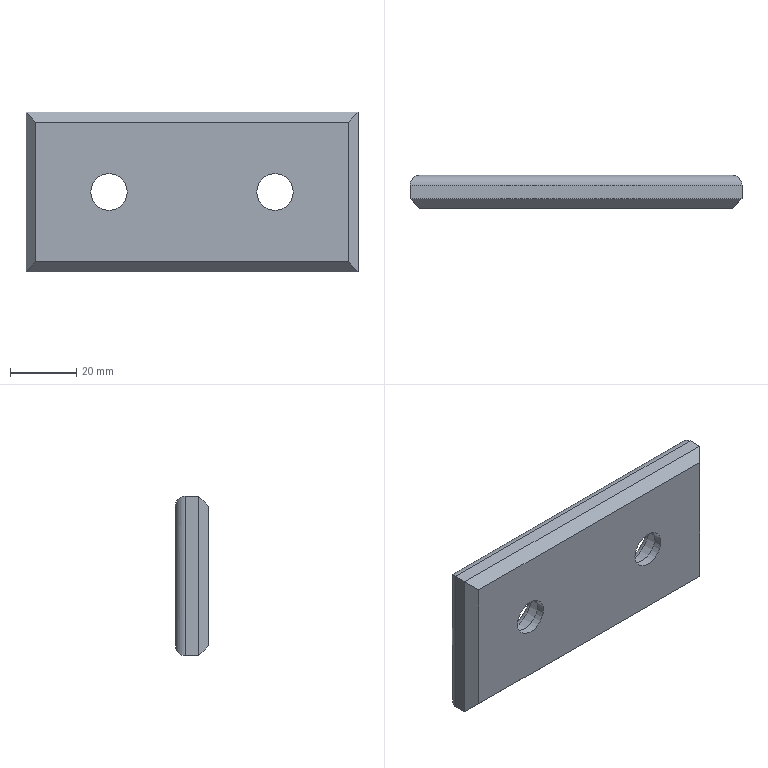Part | STEP file | lll_id4726_x_t | 1 solid | 22 faces | box 100 x 10 x 48 mm | volume 41960 mm3 | plane 12 | cylinder 8 | torus 2 | commonest cylinder face diameters 6 x4 11 x2 17.5 x2
STEP:
#1=CARTESIAN_POINT('',(1405.339,-363.359,5.));
#2=VERTEX_POINT('',#1);
#3=CARTESIAN_POINT('',(1405.339,-359.359,5.));
#4=VERTEX_POINT('',#3);
#5=CARTESIAN_POINT('',(1405.339,-361.359,5.));
#6=DIRECTION('',(0.,1.,0.));
#7=VECTOR('',#6,1.);
#8=LINE('',#5,#7);
#9=EDGE_CURVE('',#2,#4,#8,.T.);
#10=ORIENTED_EDGE('',*,*,#9,.T.);
#11=CARTESIAN_POINT('',(1305.339,-359.359,5.));
#12=VERTEX_POINT('',#11);
#13=CARTESIAN_POINT('',(1305.339,-359.359,5.));
#14=DIRECTION('',(-1.,0.,0.));
#15=VECTOR('',#14,1.);
#16=LINE('',#13,#15);
#17=EDGE_CURVE('',#4,#12,#16,.T.);
#18=ORIENTED_EDGE('',*,*,#17,.T.);
#19=CARTESIAN_POINT('',(1305.339,-363.359,5.));
#20=VERTEX_POINT('',#19);
#21=CARTESIAN_POINT('',(1305.339,-361.359,5.));
#22=DIRECTION('',(0.,-1.,0.));
#23=VECTOR('',#22,1.);
#24=LINE('',#21,#23);
#25=EDGE_CURVE('',#12,#20,#24,.T.);
#26=ORIENTED_EDGE('',*,*,#25,.T.);
#27=CARTESIAN_POINT('',(1305.339,-363.359,5.));
#28=DIRECTION('',(1.,0.,0.));
#29=VECTOR('',#28,1.);
#30=LINE('',#27,#29);
#31=EDGE_CURVE('',#20,#2,#30,.T.);
#32=ORIENTED_EDGE('',*,*,#31,.T.);
#33=EDGE_LOOP('',(#10,#18,#26,#32));
#34=FACE_OUTER_BOUND('',#33,.T.);
#35=CARTESIAN_POINT('',(1305.339,-361.359,5.));
#36=DIRECTION('',(0.,0.,1.));
#37=DIRECTION('',(-1.,0.,0.));
#38=AXIS2_PLACEMENT_3D('',#35,#36,#37);
#39=PLANE('',#38);
#40=ADVANCED_FACE('',(#34),#39,.T.);
#41=CARTESIAN_POINT('',(1405.339,-359.359,-43.));
#42=VERTEX_POINT('',#41);
#43=CARTESIAN_POINT('',(1405.339,-363.359,-43.));
#44=VERTEX_POINT('',#43);
#45=CARTESIAN_POINT('',(1405.339,-361.359,-43.));
#46=DIRECTION('',(0.,-1.,0.));
#47=VECTOR('',#46,1.);
#48=LINE('',#45,#47);
#49=EDGE_CURVE('',#42,#44,#48,.T.);
#50=ORIENTED_EDGE('',*,*,#49,.F.);
#51=CARTESIAN_POINT('',(1405.339,-359.359,-19.));
#52=DIRECTION('',(0.,0.,1.));
#53=VECTOR('',#52,1.);
#54=LINE('',#51,#53);
#55=EDGE_CURVE('',#42,#4,#54,.T.);
#56=ORIENTED_EDGE('',*,*,#55,.T.);
#57=ORIENTED_EDGE('',*,*,#9,.F.);
#58=CARTESIAN_POINT('',(1405.339,-363.359,-19.));
#59=DIRECTION('',(0.,0.,-1.));
#60=VECTOR('',#59,1.);
#61=LINE('',#58,#60);
#62=EDGE_CURVE('',#2,#44,#61,.T.);
#63=ORIENTED_EDGE('',*,*,#62,.T.);
#64=EDGE_LOOP('',(#50,#56,#57,#63));
#65=FACE_OUTER_BOUND('',#64,.T.);
#66=CARTESIAN_POINT('',(1405.339,-361.359,-19.));
#67=DIRECTION('',(1.,0.,0.));
#68=DIRECTION('',(0.,0.,1.));
#69=AXIS2_PLACEMENT_3D('',#66,#67,#68);
#70=PLANE('',#69);
#71=ADVANCED_FACE('',(#65),#70,.T.);
#72=CARTESIAN_POINT('',(1369.589,-356.359,-19.));
#73=VERTEX_POINT('',#72);
#74=CARTESIAN_POINT('',(1380.339,-356.359,-19.));
#75=DIRECTION('',(0.,-1.,0.));
#76=DIRECTION('',(-1.,0.,0.));
#77=AXIS2_PLACEMENT_3D('',#74,#75,#76);
#78=CIRCLE('',#77,10.75);
#79=EDGE_CURVE('',#73,#73,#78,.T.);
#80=ORIENTED_EDGE('',*,*,#79,.T.);
#81=EDGE_LOOP('',(#80));
#82=FACE_BOUND('',#81,.T.);
#83=CARTESIAN_POINT('',(1319.589,-356.359,-19.));
#84=VERTEX_POINT('',#83);
#85=CARTESIAN_POINT('',(1330.339,-356.359,-19.));
#86=DIRECTION('',(0.,-1.,0.));
#87=DIRECTION('',(-1.,0.,0.));
#88=AXIS2_PLACEMENT_3D('',#85,#86,#87);
#89=CIRCLE('',#88,10.75);
#90=EDGE_CURVE('',#84,#84,#89,.T.);
#91=ORIENTED_EDGE('',*,*,#90,.T.);
#92=EDGE_LOOP('',(#91));
#93=FACE_BOUND('',#92,.T.);
#94=CARTESIAN_POINT('',(1402.339,-356.359,-40.));
#95=VERTEX_POINT('',#94);
#96=CARTESIAN_POINT('',(1308.339,-356.359,-40.));
#97=VERTEX_POINT('',#96);
#98=CARTESIAN_POINT('',(1305.339,-356.359,-40.));
#99=DIRECTION('',(-1.,0.,0.));
#100=VECTOR('',#99,1.);
#101=LINE('',#98,#100);
#102=EDGE_CURVE('',#95,#97,#101,.T.);
#103=ORIENTED_EDGE('',*,*,#102,.T.);
#104=CARTESIAN_POINT('',(1308.339,-356.359,2.));
#105=VERTEX_POINT('',#104);
#106=CARTESIAN_POINT('',(1308.339,-356.359,-19.));
#107=DIRECTION('',(0.,0.,1.));
#108=VECTOR('',#107,1.);
#109=LINE('',#106,#108);
#110=EDGE_CURVE('',#97,#105,#109,.T.);
#111=ORIENTED_EDGE('',*,*,#110,.T.);
#112=CARTESIAN_POINT('',(1402.339,-356.359,2.));
#113=VERTEX_POINT('',#112);
#114=CARTESIAN_POINT('',(1305.339,-356.359,2.));
#115=DIRECTION('',(1.,0.,0.));
#116=VECTOR('',#115,1.);
#117=LINE('',#114,#116);
#118=EDGE_CURVE('',#105,#113,#117,.T.);
#119=ORIENTED_EDGE('',*,*,#118,.T.);
#120=CARTESIAN_POINT('',(1402.339,-356.359,-19.));
#121=DIRECTION('',(0.,0.,-1.));
#122=VECTOR('',#121,1.);
#123=LINE('',#120,#122);
#124=EDGE_CURVE('',#113,#95,#123,.T.);
#125=ORIENTED_EDGE('',*,*,#124,.T.);
#126=EDGE_LOOP('',(#103,#111,#119,#125));
#127=FACE_BOUND('',#126,.T.);
#128=CARTESIAN_POINT('',(1305.339,-356.359,-19.));
#129=DIRECTION('',(0.,1.,0.));
#130=DIRECTION('',(-1.,0.,0.));
#131=AXIS2_PLACEMENT_3D('',#128,#129,#130);
#132=PLANE('',#131);
#133=ADVANCED_FACE('',(#82,#93,#127),#132,.T.);
#134=CARTESIAN_POINT('',(1305.339,-363.359,-43.));
#135=VERTEX_POINT('',#134);
#136=CARTESIAN_POINT('',(1305.339,-359.359,-43.));
#137=VERTEX_POINT('',#136);
#138=CARTESIAN_POINT('',(1305.339,-361.359,-43.));
#139=DIRECTION('',(0.,1.,0.));
#140=VECTOR('',#139,1.);
#141=LINE('',#138,#140);
#142=EDGE_CURVE('',#135,#137,#141,.T.);
#143=ORIENTED_EDGE('',*,*,#142,.T.);
#144=CARTESIAN_POINT('',(1305.339,-359.359,-43.));
#145=DIRECTION('',(1.,0.,0.));
#146=VECTOR('',#145,1.);
#147=LINE('',#144,#146);
#148=EDGE_CURVE('',#137,#42,#147,.T.);
#149=ORIENTED_EDGE('',*,*,#148,.T.);
#150=ORIENTED_EDGE('',*,*,#49,.T.);
#151=CARTESIAN_POINT('',(1305.339,-363.359,-43.));
#152=DIRECTION('',(-1.,0.,0.));
#153=VECTOR('',#152,1.);
#154=LINE('',#151,#153);
#155=EDGE_CURVE('',#44,#135,#154,.T.);
#156=ORIENTED_EDGE('',*,*,#155,.T.);
#157=EDGE_LOOP('',(#143,#149,#150,#156));
#158=FACE_OUTER_BOUND('',#157,.T.);
#159=CARTESIAN_POINT('',(1305.339,-361.359,-43.));
#160=DIRECTION('',(0.,0.,-1.));
#161=DIRECTION('',(1.,0.,0.));
#162=AXIS2_PLACEMENT_3D('',#159,#160,#161);
#163=PLANE('',#162);
#164=ADVANCED_FACE('',(#158),#163,.T.);
#165=CARTESIAN_POINT('',(1374.839,-366.359,-19.));
#166=VERTEX_POINT('',#165);
#167=CARTESIAN_POINT('',(1380.339,-366.359,-19.));
#168=DIRECTION('',(0.,1.,0.));
#169=DIRECTION('',(-1.,0.,0.));
#170=AXIS2_PLACEMENT_3D('',#167,#168,#169);
#171=CIRCLE('',#170,5.5);
#172=EDGE_CURVE('',#166,#166,#171,.T.);
#173=ORIENTED_EDGE('',*,*,#172,.T.);
#174=EDGE_LOOP('',(#173));
#175=FACE_BOUND('',#174,.T.);
#176=CARTESIAN_POINT('',(1324.839,-366.359,-19.));
#177=VERTEX_POINT('',#176);
#178=CARTESIAN_POINT('',(1330.339,-366.359,-19.));
#179=DIRECTION('',(0.,1.,0.));
#180=DIRECTION('',(-1.,0.,0.));
#181=AXIS2_PLACEMENT_3D('',#178,#179,#180);
#182=CIRCLE('',#181,5.5);
#183=EDGE_CURVE('',#177,#177,#182,.T.);
#184=ORIENTED_EDGE('',*,*,#183,.T.);
#185=EDGE_LOOP('',(#184));
#186=FACE_BOUND('',#185,.T.);
#187=CARTESIAN_POINT('',(1402.339,-366.359,2.));
#188=VERTEX_POINT('',#187);
#189=CARTESIAN_POINT('',(1308.339,-366.359,2.));
#190=VERTEX_POINT('',#189);
#191=CARTESIAN_POINT('',(1305.339,-366.359,2.));
#192=DIRECTION('',(-1.,0.,0.));
#193=VECTOR('',#192,1.);
#194=LINE('',#191,#193);
#195=EDGE_CURVE('',#188,#190,#194,.T.);
#196=ORIENTED_EDGE('',*,*,#195,.T.);
#197=CARTESIAN_POINT('',(1308.339,-366.359,-40.));
#198=VERTEX_POINT('',#197);
#199=CARTESIAN_POINT('',(1308.339,-366.359,-19.));
#200=DIRECTION('',(0.,0.,-1.));
#201=VECTOR('',#200,1.);
#202=LINE('',#199,#201);
#203=EDGE_CURVE('',#190,#198,#202,.T.);
#204=ORIENTED_EDGE('',*,*,#203,.T.);
#205=CARTESIAN_POINT('',(1402.339,-366.359,-40.));
#206=VERTEX_POINT('',#205);
#207=CARTESIAN_POINT('',(1305.339,-366.359,-40.));
#208=DIRECTION('',(1.,0.,0.));
#209=VECTOR('',#208,1.);
#210=LINE('',#207,#209);
#211=EDGE_CURVE('',#198,#206,#210,.T.);
#212=ORIENTED_EDGE('',*,*,#211,.T.);
#213=CARTESIAN_POINT('',(1402.339,-366.359,-19.));
#214=DIRECTION('',(0.,0.,1.));
#215=VECTOR('',#214,1.);
#216=LINE('',#213,#215);
#217=EDGE_CURVE('',#206,#188,#216,.T.);
#218=ORIENTED_EDGE('',*,*,#217,.T.);
#219=EDGE_LOOP('',(#196,#204,#212,#218));
#220=FACE_BOUND('',#219,.T.);
#221=CARTESIAN_POINT('',(1305.339,-366.359,-19.));
#222=DIRECTION('',(0.,-1.,0.));
#223=DIRECTION('',(1.,0.,0.));
#224=AXIS2_PLACEMENT_3D('',#221,#222,#223);
#225=PLANE('',#224);
#226=ADVANCED_FACE('',(#175,#186,#220),#225,.T.);
#227=ORIENTED_EDGE('',*,*,#25,.F.);
#228=CARTESIAN_POINT('',(1305.339,-359.359,-19.));
#229=DIRECTION('',(0.,0.,-1.));
#230=VECTOR('',#229,1.);
#231=LINE('',#228,#230);
#232=EDGE_CURVE('',#12,#137,#231,.T.);
#233=ORIENTED_EDGE('',*,*,#232,.T.);
#234=ORIENTED_EDGE('',*,*,#142,.F.);
#235=CARTESIAN_POINT('',(1305.339,-363.359,-19.));
#236=DIRECTION('',(0.,0.,1.));
#237=VECTOR('',#236,1.);
#238=LINE('',#235,#237);
#239=EDGE_CURVE('',#135,#20,#238,.T.);
#240=ORIENTED_EDGE('',*,*,#239,.T.);
#241=EDGE_LOOP('',(#227,#233,#234,#240));
#242=FACE_OUTER_BOUND('',#241,.T.);
#243=CARTESIAN_POINT('',(1305.339,-361.359,-19.));
#244=DIRECTION('',(-1.,0.,0.));
#245=DIRECTION('',(0.,0.,-1.));
#246=AXIS2_PLACEMENT_3D('',#243,#244,#245);
#247=PLANE('',#246);
#248=ADVANCED_FACE('',(#242),#247,.T.);
#249=CARTESIAN_POINT('',(1395.339,-373.359,-33.));
#250=DIRECTION('',(-0.5774,-0.5774,0.5774));
#251=VECTOR('',#250,1.);
#252=LINE('',#249,#251);
#253=EDGE_CURVE('',#44,#206,#252,.T.);
#254=ORIENTED_EDGE('',*,*,#253,.F.);
#255=ORIENTED_EDGE('',*,*,#62,.F.);
#256=CARTESIAN_POINT('',(1395.339,-373.359,-5.));
#257=DIRECTION('',(0.5774,0.5774,0.5774));
#258=VECTOR('',#257,1.);
#259=LINE('',#256,#258);
#260=EDGE_CURVE('',#188,#2,#259,.T.);
#261=ORIENTED_EDGE('',*,*,#260,.F.);
#262=ORIENTED_EDGE('',*,*,#217,.F.);
#263=EDGE_LOOP('',(#254,#255,#261,#262));
#264=FACE_OUTER_BOUND('',#263,.T.);
#265=CARTESIAN_POINT('',(1402.339,-366.359,-19.));
#266=DIRECTION('',(-0.7071,0.7071,0.));
#267=DIRECTION('',(-0.7071,-0.7071,0.));
#268=AXIS2_PLACEMENT_3D('',#265,#266,#267);
#269=PLANE('',#268);
#270=ADVANCED_FACE('',(#264),#269,.F.);
#271=ORIENTED_EDGE('',*,*,#260,.T.);
#272=ORIENTED_EDGE('',*,*,#31,.F.);
#273=CARTESIAN_POINT('',(1305.339,-363.359,5.));
#274=DIRECTION('',(-0.5774,0.5774,0.5774));
#275=VECTOR('',#274,1.);
#276=LINE('',#273,#275);
#277=EDGE_CURVE('',#190,#20,#276,.T.);
#278=ORIENTED_EDGE('',*,*,#277,.F.);
#279=ORIENTED_EDGE('',*,*,#195,.F.);
#280=EDGE_LOOP('',(#271,#272,#278,#279));
#281=FACE_OUTER_BOUND('',#280,.T.);
#282=CARTESIAN_POINT('',(1305.339,-363.359,5.));
#283=DIRECTION('',(0.,0.7071,-0.7071));
#284=DIRECTION('',(0.,0.7071,0.7071));
#285=AXIS2_PLACEMENT_3D('',#282,#283,#284);
#286=PLANE('',#285);
#287=ADVANCED_FACE('',(#281),#286,.F.);
#288=ORIENTED_EDGE('',*,*,#253,.T.);
#289=ORIENTED_EDGE('',*,*,#211,.F.);
#290=CARTESIAN_POINT('',(1307.339,-365.359,-41.));
#291=DIRECTION('',(0.5774,-0.5774,0.5774));
#292=VECTOR('',#291,1.);
#293=LINE('',#290,#292);
#294=EDGE_CURVE('',#135,#198,#293,.T.);
#295=ORIENTED_EDGE('',*,*,#294,.F.);
#296=ORIENTED_EDGE('',*,*,#155,.F.);
#297=EDGE_LOOP('',(#288,#289,#295,#296));
#298=FACE_OUTER_BOUND('',#297,.T.);
#299=CARTESIAN_POINT('',(1305.339,-366.359,-40.));
#300=DIRECTION('',(0.,0.7071,0.7071));
#301=DIRECTION('',(0.,-0.7071,0.7071));
#302=AXIS2_PLACEMENT_3D('',#299,#300,#301);
#303=PLANE('',#302);
#304=ADVANCED_FACE('',(#298),#303,.F.);
#305=ORIENTED_EDGE('',*,*,#277,.T.);
#306=ORIENTED_EDGE('',*,*,#239,.F.);
#307=ORIENTED_EDGE('',*,*,#294,.T.);
#308=ORIENTED_EDGE('',*,*,#203,.F.);
#309=EDGE_LOOP('',(#305,#306,#307,#308));
#310=FACE_OUTER_BOUND('',#309,.T.);
#311=CARTESIAN_POINT('',(1308.339,-366.359,-19.));
#312=DIRECTION('',(0.7071,0.7071,0.));
#313=DIRECTION('',(-0.7071,0.7071,0.));
#314=AXIS2_PLACEMENT_3D('',#311,#312,#313);
#315=PLANE('',#314);
#316=ADVANCED_FACE('',(#310),#315,.F.);
#317=CARTESIAN_POINT('',(1402.339,-359.359,2.));
#318=DIRECTION('',(-0.7071,0.,0.7071));
#319=DIRECTION('',(-0.7071,0.,-0.7071));
#320=AXIS2_PLACEMENT_3D('',#317,#318,#319);
#321=ELLIPSE('',#320,4.243,3.);
#322=EDGE_CURVE('',#4,#113,#321,.T.);
#323=ORIENTED_EDGE('',*,*,#322,.F.);
#324=ORIENTED_EDGE('',*,*,#55,.F.);
#325=CARTESIAN_POINT('',(1402.339,-359.359,-40.));
#326=DIRECTION('',(-0.7071,0.,-0.7071));
#327=DIRECTION('',(0.7071,0.,-0.7071));
#328=AXIS2_PLACEMENT_3D('',#325,#326,#327);
#329=ELLIPSE('',#328,4.243,3.);
#330=EDGE_CURVE('',#95,#42,#329,.T.);
#331=ORIENTED_EDGE('',*,*,#330,.F.);
#332=ORIENTED_EDGE('',*,*,#124,.F.);
#333=EDGE_LOOP('',(#323,#324,#331,#332));
#334=FACE_OUTER_BOUND('',#333,.T.);
#335=CARTESIAN_POINT('',(1402.339,-359.359,-19.));
#336=DIRECTION('',(0.,0.,-1.));
#337=DIRECTION('',(1.,0.,0.));
#338=AXIS2_PLACEMENT_3D('',#335,#336,#337);
#339=CYLINDRICAL_SURFACE('',#338,3.);
#340=ADVANCED_FACE('',(#334),#339,.T.);
#341=ORIENTED_EDGE('',*,*,#330,.T.);
#342=ORIENTED_EDGE('',*,*,#148,.F.);
#343=CARTESIAN_POINT('',(1308.339,-359.359,-40.));
#344=DIRECTION('',(-0.7071,0.,0.7071));
#345=DIRECTION('',(0.7071,0.,0.7071));
#346=AXIS2_PLACEMENT_3D('',#343,#344,#345);
#347=ELLIPSE('',#346,4.243,3.);
#348=EDGE_CURVE('',#97,#137,#347,.T.);
#349=ORIENTED_EDGE('',*,*,#348,.F.);
#350=ORIENTED_EDGE('',*,*,#102,.F.);
#351=EDGE_LOOP('',(#341,#342,#349,#350));
#352=FACE_OUTER_BOUND('',#351,.T.);
#353=CARTESIAN_POINT('',(1305.339,-359.359,-40.));
#354=DIRECTION('',(1.,0.,0.));
#355=DIRECTION('',(0.,0.,1.));
#356=AXIS2_PLACEMENT_3D('',#353,#354,#355);
#357=CYLINDRICAL_SURFACE('',#356,3.);
#358=ADVANCED_FACE('',(#352),#357,.T.);
#359=ORIENTED_EDGE('',*,*,#322,.T.);
#360=ORIENTED_EDGE('',*,*,#118,.F.);
#361=CARTESIAN_POINT('',(1308.339,-359.359,2.));
#362=DIRECTION('',(-0.7071,0.,-0.7071));
#363=DIRECTION('',(0.7071,0.,-0.7071));
#364=AXIS2_PLACEMENT_3D('',#361,#362,#363);
#365=ELLIPSE('',#364,4.243,3.);
#366=EDGE_CURVE('',#12,#105,#365,.T.);
#367=ORIENTED_EDGE('',*,*,#366,.F.);
#368=ORIENTED_EDGE('',*,*,#17,.F.);
#369=EDGE_LOOP('',(#359,#360,#367,#368));
#370=FACE_OUTER_BOUND('',#369,.T.);
#371=CARTESIAN_POINT('',(1305.339,-359.359,2.));
#372=DIRECTION('',(1.,0.,0.));
#373=DIRECTION('',(0.,0.,1.));
#374=AXIS2_PLACEMENT_3D('',#371,#372,#373);
#375=CYLINDRICAL_SURFACE('',#374,3.);
#376=ADVANCED_FACE('',(#370),#375,.T.);
#377=ORIENTED_EDGE('',*,*,#348,.T.);
#378=ORIENTED_EDGE('',*,*,#232,.F.);
#379=ORIENTED_EDGE('',*,*,#366,.T.);
#380=ORIENTED_EDGE('',*,*,#110,.F.);
#381=EDGE_LOOP('',(#377,#378,#379,#380));
#382=FACE_OUTER_BOUND('',#381,.T.);
#383=CARTESIAN_POINT('',(1308.339,-359.359,-19.));
#384=DIRECTION('',(0.,0.,1.));
#385=DIRECTION('',(-1.,0.,0.));
#386=AXIS2_PLACEMENT_3D('',#383,#384,#385);
#387=CYLINDRICAL_SURFACE('',#386,3.);
#388=ADVANCED_FACE('',(#382),#387,.T.);
#389=CARTESIAN_POINT('',(1335.839,-363.859,-19.));
#390=VERTEX_POINT('',#389);
#391=CARTESIAN_POINT('',(1330.339,-363.859,-19.));
#392=DIRECTION('',(0.,-1.,0.));
#393=DIRECTION('',(1.,0.,0.));
#394=AXIS2_PLACEMENT_3D('',#391,#392,#393);
#395=CIRCLE('',#394,5.5);
#396=EDGE_CURVE('',#390,#390,#395,.T.);
#397=ORIENTED_EDGE('',*,*,#396,.T.);
#398=EDGE_LOOP('',(#397));
#399=FACE_BOUND('',#398,.T.);
#400=CARTESIAN_POINT('',(1321.589,-363.859,-19.));
#401=VERTEX_POINT('',#400);
#402=CARTESIAN_POINT('',(1330.339,-363.859,-19.));
#403=DIRECTION('',(0.,-1.,0.));
#404=DIRECTION('',(-1.,0.,0.));
#405=AXIS2_PLACEMENT_3D('',#402,#403,#404);
#406=CIRCLE('',#405,8.75);
#407=EDGE_CURVE('',#401,#401,#406,.T.);
#408=ORIENTED_EDGE('',*,*,#407,.F.);
#409=EDGE_LOOP('',(#408));
#410=FACE_BOUND('',#409,.T.);
#411=CARTESIAN_POINT('',(1330.339,-363.859,-19.));
#412=DIRECTION('',(0.,-1.,0.));
#413=DIRECTION('',(1.,0.,0.));
#414=AXIS2_PLACEMENT_3D('',#411,#412,#413);
#415=PLANE('',#414);
#416=ADVANCED_FACE('',(#399,#410),#415,.F.);
#417=CARTESIAN_POINT('',(1321.589,-358.359,-19.));
#418=VERTEX_POINT('',#417);
#419=CARTESIAN_POINT('',(1330.339,-358.359,-19.));
#420=DIRECTION('',(0.,1.,0.));
#421=DIRECTION('',(-1.,0.,0.));
#422=AXIS2_PLACEMENT_3D('',#419,#420,#421);
#423=CIRCLE('',#422,8.75);
#424=EDGE_CURVE('',#418,#418,#423,.T.);
#425=ORIENTED_EDGE('',*,*,#424,.T.);
#426=EDGE_LOOP('',(#425));
#427=FACE_BOUND('',#426,.T.);
#428=ORIENTED_EDGE('',*,*,#407,.T.);
#429=EDGE_LOOP('',(#428));
#430=FACE_BOUND('',#429,.T.);
#431=CARTESIAN_POINT('',(1330.339,-356.359,-19.));
#432=DIRECTION('',(0.,-1.,0.));
#433=DIRECTION('',(1.,0.,0.));
#434=AXIS2_PLACEMENT_3D('',#431,#432,#433);
#435=CYLINDRICAL_SURFACE('',#434,8.75);
#436=ADVANCED_FACE('',(#427,#430),#435,.F.);
#437=ORIENTED_EDGE('',*,*,#183,.F.);
#438=EDGE_LOOP('',(#437));
#439=FACE_BOUND('',#438,.T.);
#440=ORIENTED_EDGE('',*,*,#396,.F.);
#441=EDGE_LOOP('',(#440));
#442=FACE_BOUND('',#441,.T.);
#443=CARTESIAN_POINT('',(1330.339,-356.359,-19.));
#444=DIRECTION('',(0.,-1.,0.));
#445=DIRECTION('',(1.,0.,0.));
#446=AXIS2_PLACEMENT_3D('',#443,#444,#445);
#447=CYLINDRICAL_SURFACE('',#446,5.5);
#448=ADVANCED_FACE('',(#439,#442),#447,.F.);
#449=CARTESIAN_POINT('',(1385.839,-363.859,-19.));
#450=VERTEX_POINT('',#449);
#451=CARTESIAN_POINT('',(1380.339,-363.859,-19.));
#452=DIRECTION('',(0.,-1.,0.));
#453=DIRECTION('',(1.,0.,0.));
#454=AXIS2_PLACEMENT_3D('',#451,#452,#453);
#455=CIRCLE('',#454,5.5);
#456=EDGE_CURVE('',#450,#450,#455,.T.);
#457=ORIENTED_EDGE('',*,*,#456,.T.);
#458=EDGE_LOOP('',(#457));
#459=FACE_BOUND('',#458,.T.);
#460=CARTESIAN_POINT('',(1371.589,-363.859,-19.));
#461=VERTEX_POINT('',#460);
#462=CARTESIAN_POINT('',(1380.339,-363.859,-19.));
#463=DIRECTION('',(0.,-1.,0.));
#464=DIRECTION('',(-1.,0.,0.));
#465=AXIS2_PLACEMENT_3D('',#462,#463,#464);
#466=CIRCLE('',#465,8.75);
#467=EDGE_CURVE('',#461,#461,#466,.T.);
#468=ORIENTED_EDGE('',*,*,#467,.F.);
#469=EDGE_LOOP('',(#468));
#470=FACE_BOUND('',#469,.T.);
#471=CARTESIAN_POINT('',(1380.339,-363.859,-19.));
#472=DIRECTION('',(0.,-1.,0.));
#473=DIRECTION('',(1.,0.,0.));
#474=AXIS2_PLACEMENT_3D('',#471,#472,#473);
#475=PLANE('',#474);
#476=ADVANCED_FACE('',(#459,#470),#475,.F.);
#477=CARTESIAN_POINT('',(1371.589,-358.359,-19.));
#478=VERTEX_POINT('',#477);
#479=CARTESIAN_POINT('',(1380.339,-358.359,-19.));
#480=DIRECTION('',(0.,1.,0.));
#481=DIRECTION('',(-1.,0.,0.));
#482=AXIS2_PLACEMENT_3D('',#479,#480,#481);
#483=CIRCLE('',#482,8.75);
#484=EDGE_CURVE('',#478,#478,#483,.T.);
#485=ORIENTED_EDGE('',*,*,#484,.T.);
#486=EDGE_LOOP('',(#485));
#487=FACE_BOUND('',#486,.T.);
#488=ORIENTED_EDGE('',*,*,#467,.T.);
#489=EDGE_LOOP('',(#488));
#490=FACE_BOUND('',#489,.T.);
#491=CARTESIAN_POINT('',(1380.339,-356.359,-19.));
#492=DIRECTION('',(0.,-1.,0.));
#493=DIRECTION('',(1.,0.,0.));
#494=AXIS2_PLACEMENT_3D('',#491,#492,#493);
#495=CYLINDRICAL_SURFACE('',#494,8.75);
#496=ADVANCED_FACE('',(#487,#490),#495,.F.);
#497=ORIENTED_EDGE('',*,*,#172,.F.);
#498=EDGE_LOOP('',(#497));
#499=FACE_BOUND('',#498,.T.);
#500=ORIENTED_EDGE('',*,*,#456,.F.);
#501=EDGE_LOOP('',(#500));
#502=FACE_BOUND('',#501,.T.);
#503=CARTESIAN_POINT('',(1380.339,-356.359,-19.));
#504=DIRECTION('',(0.,-1.,0.));
#505=DIRECTION('',(1.,0.,0.));
#506=AXIS2_PLACEMENT_3D('',#503,#504,#505);
#507=CYLINDRICAL_SURFACE('',#506,5.5);
#508=ADVANCED_FACE('',(#499,#502),#507,.F.);
#509=ORIENTED_EDGE('',*,*,#424,.F.);
#510=EDGE_LOOP('',(#509));
#511=FACE_BOUND('',#510,.T.);
#512=ORIENTED_EDGE('',*,*,#90,.F.);
#513=EDGE_LOOP('',(#512));
#514=FACE_BOUND('',#513,.T.);
#515=CARTESIAN_POINT('',(1330.339,-358.359,-19.));
#516=DIRECTION('',(0.,1.,0.));
#517=DIRECTION('',(-1.,0.,0.));
#518=AXIS2_PLACEMENT_3D('',#515,#516,#517);
#519=TOROIDAL_SURFACE('',#518,10.75,2.);
#520=ADVANCED_FACE('',(#511,#514),#519,.T.);
#521=ORIENTED_EDGE('',*,*,#484,.F.);
#522=EDGE_LOOP('',(#521));
#523=FACE_BOUND('',#522,.T.);
#524=ORIENTED_EDGE('',*,*,#79,.F.);
#525=EDGE_LOOP('',(#524));
#526=FACE_BOUND('',#525,.T.);
#527=CARTESIAN_POINT('',(1380.339,-358.359,-19.));
#528=DIRECTION('',(0.,1.,0.));
#529=DIRECTION('',(-1.,0.,0.));
#530=AXIS2_PLACEMENT_3D('',#527,#528,#529);
#531=TOROIDAL_SURFACE('',#530,10.75,2.);
#532=ADVANCED_FACE('',(#523,#526),#531,.T.);
#533=CLOSED_SHELL('',(#40,#71,#133,#164,#226,#248,#270,#287,#304,#316,#340,#358,#376,#388,#416,#436,#448,#476,#496,#508,#520,#532));
#534=MANIFOLD_SOLID_BREP('',#533);
#535=(LENGTH_UNIT()NAMED_UNIT(*)SI_UNIT(.MILLI.,.METRE.));
#536=UNCERTAINTY_MEASURE_WITH_UNIT(LENGTH_MEASURE(0.00002),#535,'','');
#537=(NAMED_UNIT(*)PLANE_ANGLE_UNIT()SI_UNIT($,.RADIAN.));
#538=PLANE_ANGLE_MEASURE_WITH_UNIT(PLANE_ANGLE_MEASURE(0.01745),#537);
#539=DIMENSIONAL_EXPONENTS(0.,0.,0.,0.,0.,0.,0.);
#540=(CONVERSION_BASED_UNIT('DEGREE',#538)NAMED_UNIT(#539)PLANE_ANGLE_UNIT());
#541=(NAMED_UNIT(*)SI_UNIT($,.STERADIAN.)SOLID_ANGLE_UNIT());
#542=(GEOMETRIC_REPRESENTATION_CONTEXT(3)GLOBAL_UNCERTAINTY_ASSIGNED_CONTEXT((#536))GLOBAL_UNIT_ASSIGNED_CONTEXT((#535,#540,#541))REPRESENTATION_CONTEXT('',''));
#543=ADVANCED_BREP_SHAPE_REPRESENTATION('',(#534),#542);